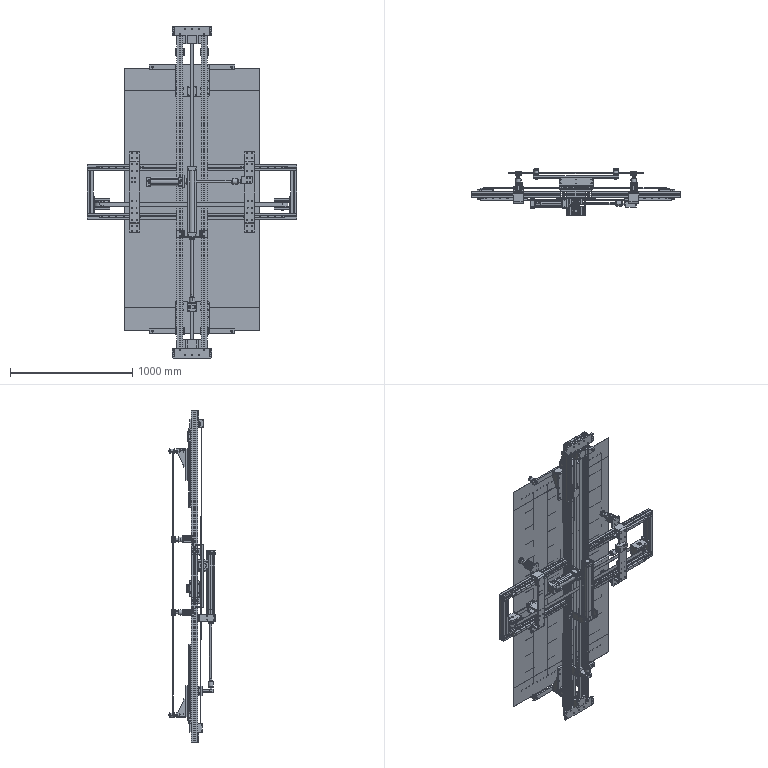Part | SolidWorks | features ReferencePattern 10, LocalLPattern 2, AEMSimFeature 1, CompositeCurve 1 | 184 solids | 10319 faces | volume 38951088 mm3 | plane 4547 | cylinder 3766 | torus 882 | cone 606 | sphere 472 | spline 46 | commonest cylinder face diameters 5 x380 1 x344 11 x280 1.2 x240 9 x220 7 x190